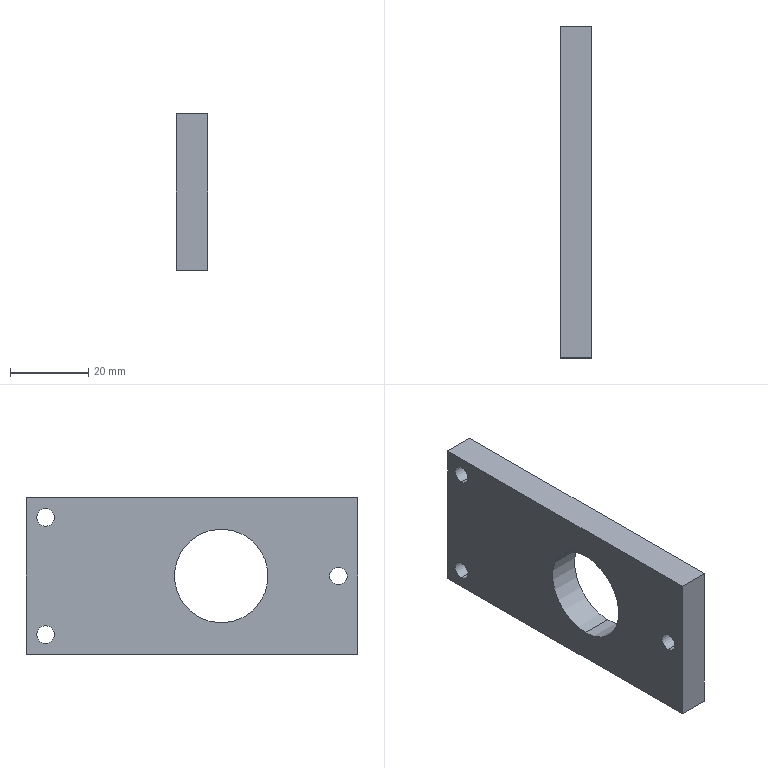Part | STEP file | 0243_213_Plate | 1 solid | 14 faces | box 8 x 85 x 40 mm | volume 23199 mm3 | cylinder 8 | plane 6 | commonest cylinder face diameters 4.5 x6 24 x2
STEP:
#1=CARTESIAN_POINT('',(0.,0.,0.));
#2=DIRECTION('',(0.,0.,1.));
#3=DIRECTION('',(1.,0.,0.));
#4=AXIS2_PLACEMENT_3D('',#1,#2,#3);
#5=CARTESIAN_POINT('',(0.,-80.,-2.25));
#6=VERTEX_POINT('',#5);
#7=CARTESIAN_POINT('',(8.,-80.,-2.25));
#8=VERTEX_POINT('',#7);
#9=CARTESIAN_POINT('',(8.,-80.,-2.25));
#10=DIRECTION('',(1.,0.,0.));
#11=VECTOR('',#10,1.);
#12=LINE('',#9,#11);
#13=CARTESIAN_POINT('',(8.,-80.,0.));
#14=DIRECTION('',(1.,0.,0.));
#15=DIRECTION('',(0.,0.,-1.));
#16=AXIS2_PLACEMENT_3D('',#13,#14,#15);
#17=CYLINDRICAL_SURFACE('',#16,2.25);
#18=CARTESIAN_POINT('',(6.283,0.));
#19=DIRECTION('',(0.,1.));
#20=VECTOR('',#19,1.);
#21=LINE('',#18,#20);
#22=(GEOMETRIC_REPRESENTATION_CONTEXT(2)PARAMETRIC_REPRESENTATION_CONTEXT()REPRESENTATION_CONTEXT('',''));
#23=DEFINITIONAL_REPRESENTATION('',(#21),#22);
#24=PCURVE('',#17,#23);
#25=CARTESIAN_POINT('',(8.,-80.,0.));
#26=DIRECTION('',(1.,0.,0.));
#27=DIRECTION('',(0.,0.,-1.));
#28=AXIS2_PLACEMENT_3D('',#25,#26,#27);
#29=CYLINDRICAL_SURFACE('',#28,2.25);
#30=CARTESIAN_POINT('',(0.,0.));
#31=DIRECTION('',(0.,1.));
#32=VECTOR('',#31,1.);
#33=LINE('',#30,#32);
#34=(GEOMETRIC_REPRESENTATION_CONTEXT(2)PARAMETRIC_REPRESENTATION_CONTEXT()REPRESENTATION_CONTEXT('',''));
#35=DEFINITIONAL_REPRESENTATION('',(#33),#34);
#36=PCURVE('',#29,#35);
#37=SURFACE_CURVE('',#12,(#24,#36),.PCURVE_S1.);
#38=EDGE_CURVE('',#6,#8,#37,.T.);
#39=ORIENTED_EDGE('',*,*,#38,.T.);
#40=CARTESIAN_POINT('',(8.,-80.,2.25));
#41=VERTEX_POINT('',#40);
#42=CARTESIAN_POINT('',(8.,-80.,0.));
#43=DIRECTION('',(1.,0.,0.));
#44=DIRECTION('',(0.,0.,-1.));
#45=AXIS2_PLACEMENT_3D('',#42,#43,#44);
#46=CIRCLE('',#45,2.25);
#47=CARTESIAN_POINT('',(0.,0.));
#48=DIRECTION('',(1.,0.));
#49=VECTOR('',#48,1.);
#50=LINE('',#47,#49);
#51=(GEOMETRIC_REPRESENTATION_CONTEXT(2)PARAMETRIC_REPRESENTATION_CONTEXT()REPRESENTATION_CONTEXT('',''));
#52=DEFINITIONAL_REPRESENTATION('',(#50),#51);
#53=PCURVE('',#17,#52);
#54=CARTESIAN_POINT('',(8.,0.,20.));
#55=DIRECTION('',(-1.,0.,0.));
#56=DIRECTION('',(0.,0.,1.));
#57=AXIS2_PLACEMENT_3D('',#54,#55,#56);
#58=PLANE('',#57);
#59=CARTESIAN_POINT('',(-22.25,-80.));
#60=CARTESIAN_POINT('',(-22.25,-76.103));
#61=CARTESIAN_POINT('',(-18.875,-78.051));
#62=CARTESIAN_POINT('',(-15.5,-80.));
#63=CARTESIAN_POINT('',(-18.875,-81.949));
#64=CARTESIAN_POINT('',(-22.25,-83.897));
#65=CARTESIAN_POINT('',(-22.25,-80.));
#66=(BOUNDED_CURVE()B_SPLINE_CURVE(2,(#59,#60,#61,#62,#63,#64,#65),.UNSPECIFIED.,.T.,.F.)B_SPLINE_CURVE_WITH_KNOTS((1,2,2,2,2,1),(-2.094,0.,2.094,4.189,6.283,8.378),.UNSPECIFIED.)CURVE()GEOMETRIC_REPRESENTATION_ITEM()RATIONAL_B_SPLINE_CURVE((1.,0.5,1.,0.5,1.,0.5,1.))REPRESENTATION_ITEM(''));
#67=(GEOMETRIC_REPRESENTATION_CONTEXT(2)PARAMETRIC_REPRESENTATION_CONTEXT()REPRESENTATION_CONTEXT('',''));
#68=DEFINITIONAL_REPRESENTATION('',(#66),#67);
#69=PCURVE('',#58,#68);
#70=SURFACE_CURVE('',#46,(#53,#69),.PCURVE_S1.);
#71=EDGE_CURVE('',#41,#8,#70,.T.);
#72=ORIENTED_EDGE('',*,*,#71,.F.);
#73=CARTESIAN_POINT('',(0.,-80.,2.25));
#74=VERTEX_POINT('',#73);
#75=CARTESIAN_POINT('',(8.,-80.,2.25));
#76=DIRECTION('',(1.,0.,0.));
#77=VECTOR('',#76,1.);
#78=LINE('',#75,#77);
#79=CARTESIAN_POINT('',(3.142,0.));
#80=DIRECTION('',(0.,1.));
#81=VECTOR('',#80,1.);
#82=LINE('',#79,#81);
#83=(GEOMETRIC_REPRESENTATION_CONTEXT(2)PARAMETRIC_REPRESENTATION_CONTEXT()REPRESENTATION_CONTEXT('',''));
#84=DEFINITIONAL_REPRESENTATION('',(#82),#83);
#85=PCURVE('',#17,#84);
#86=CARTESIAN_POINT('',(3.142,0.));
#87=DIRECTION('',(0.,1.));
#88=VECTOR('',#87,1.);
#89=LINE('',#86,#88);
#90=(GEOMETRIC_REPRESENTATION_CONTEXT(2)PARAMETRIC_REPRESENTATION_CONTEXT()REPRESENTATION_CONTEXT('',''));
#91=DEFINITIONAL_REPRESENTATION('',(#89),#90);
#92=PCURVE('',#29,#91);
#93=SURFACE_CURVE('',#78,(#85,#92),.PCURVE_S1.);
#94=EDGE_CURVE('',#74,#41,#93,.T.);
#95=ORIENTED_EDGE('',*,*,#94,.F.);
#96=CARTESIAN_POINT('',(0.,-80.,0.));
#97=DIRECTION('',(1.,0.,0.));
#98=DIRECTION('',(0.,0.,-1.));
#99=AXIS2_PLACEMENT_3D('',#96,#97,#98);
#100=CIRCLE('',#99,2.25);
#101=CARTESIAN_POINT('',(0.,-8.));
#102=DIRECTION('',(1.,0.));
#103=VECTOR('',#102,1.);
#104=LINE('',#101,#103);
#105=(GEOMETRIC_REPRESENTATION_CONTEXT(2)PARAMETRIC_REPRESENTATION_CONTEXT()REPRESENTATION_CONTEXT('',''));
#106=DEFINITIONAL_REPRESENTATION('',(#104),#105);
#107=PCURVE('',#17,#106);
#108=CARTESIAN_POINT('',(0.,0.,20.));
#109=DIRECTION('',(-1.,0.,0.));
#110=DIRECTION('',(0.,0.,1.));
#111=AXIS2_PLACEMENT_3D('',#108,#109,#110);
#112=PLANE('',#111);
#113=CARTESIAN_POINT('',(-22.25,-80.));
#114=CARTESIAN_POINT('',(-22.25,-76.103));
#115=CARTESIAN_POINT('',(-18.875,-78.051));
#116=CARTESIAN_POINT('',(-15.5,-80.));
#117=CARTESIAN_POINT('',(-18.875,-81.949));
#118=CARTESIAN_POINT('',(-22.25,-83.897));
#119=CARTESIAN_POINT('',(-22.25,-80.));
#120=(BOUNDED_CURVE()B_SPLINE_CURVE(2,(#113,#114,#115,#116,#117,#118,#119),.UNSPECIFIED.,.T.,.F.)B_SPLINE_CURVE_WITH_KNOTS((1,2,2,2,2,1),(-2.094,0.,2.094,4.189,6.283,8.378),.UNSPECIFIED.)CURVE()GEOMETRIC_REPRESENTATION_ITEM()RATIONAL_B_SPLINE_CURVE((1.,0.5,1.,0.5,1.,0.5,1.))REPRESENTATION_ITEM(''));
#121=(GEOMETRIC_REPRESENTATION_CONTEXT(2)PARAMETRIC_REPRESENTATION_CONTEXT()REPRESENTATION_CONTEXT('',''));
#122=DEFINITIONAL_REPRESENTATION('',(#120),#121);
#123=PCURVE('',#112,#122);
#124=SURFACE_CURVE('',#100,(#107,#123),.PCURVE_S1.);
#125=EDGE_CURVE('',#74,#6,#124,.T.);
#126=ORIENTED_EDGE('',*,*,#125,.T.);
#127=EDGE_LOOP('',(#39,#72,#95,#126));
#128=FACE_BOUND('',#127,.F.);
#129=ADVANCED_FACE('',(#128),#17,.F.);
#130=CARTESIAN_POINT('',(0.,-5.,12.75));
#131=VERTEX_POINT('',#130);
#132=CARTESIAN_POINT('',(8.,-5.,12.75));
#133=VERTEX_POINT('',#132);
#134=CARTESIAN_POINT('',(8.,-5.,12.75));
#135=DIRECTION('',(1.,0.,0.));
#136=VECTOR('',#135,1.);
#137=LINE('',#134,#136);
#138=CARTESIAN_POINT('',(8.,-5.,15.));
#139=DIRECTION('',(1.,0.,0.));
#140=DIRECTION('',(0.,0.,-1.));
#141=AXIS2_PLACEMENT_3D('',#138,#139,#140);
#142=CYLINDRICAL_SURFACE('',#141,2.25);
#143=CARTESIAN_POINT('',(6.283,0.));
#144=DIRECTION('',(0.,1.));
#145=VECTOR('',#144,1.);
#146=LINE('',#143,#145);
#147=(GEOMETRIC_REPRESENTATION_CONTEXT(2)PARAMETRIC_REPRESENTATION_CONTEXT()REPRESENTATION_CONTEXT('',''));
#148=DEFINITIONAL_REPRESENTATION('',(#146),#147);
#149=PCURVE('',#142,#148);
#150=CARTESIAN_POINT('',(8.,-5.,15.));
#151=DIRECTION('',(1.,0.,0.));
#152=DIRECTION('',(0.,0.,-1.));
#153=AXIS2_PLACEMENT_3D('',#150,#151,#152);
#154=CYLINDRICAL_SURFACE('',#153,2.25);
#155=CARTESIAN_POINT('',(0.,0.));
#156=DIRECTION('',(0.,1.));
#157=VECTOR('',#156,1.);
#158=LINE('',#155,#157);
#159=(GEOMETRIC_REPRESENTATION_CONTEXT(2)PARAMETRIC_REPRESENTATION_CONTEXT()REPRESENTATION_CONTEXT('',''));
#160=DEFINITIONAL_REPRESENTATION('',(#158),#159);
#161=PCURVE('',#154,#160);
#162=SURFACE_CURVE('',#137,(#149,#161),.PCURVE_S1.);
#163=EDGE_CURVE('',#131,#133,#162,.T.);
#164=ORIENTED_EDGE('',*,*,#163,.T.);
#165=CARTESIAN_POINT('',(8.,-5.,17.25));
#166=VERTEX_POINT('',#165);
#167=CARTESIAN_POINT('',(8.,-5.,15.));
#168=DIRECTION('',(1.,0.,0.));
#169=DIRECTION('',(0.,0.,-1.));
#170=AXIS2_PLACEMENT_3D('',#167,#168,#169);
#171=CIRCLE('',#170,2.25);
#172=CARTESIAN_POINT('',(0.,0.));
#173=DIRECTION('',(1.,0.));
#174=VECTOR('',#173,1.);
#175=LINE('',#172,#174);
#176=(GEOMETRIC_REPRESENTATION_CONTEXT(2)PARAMETRIC_REPRESENTATION_CONTEXT()REPRESENTATION_CONTEXT('',''));
#177=DEFINITIONAL_REPRESENTATION('',(#175),#176);
#178=PCURVE('',#142,#177);
#179=CARTESIAN_POINT('',(-7.25,-5.));
#180=CARTESIAN_POINT('',(-7.25,-1.103));
#181=CARTESIAN_POINT('',(-3.875,-3.051));
#182=CARTESIAN_POINT('',(-0.5,-5.));
#183=CARTESIAN_POINT('',(-3.875,-6.949));
#184=CARTESIAN_POINT('',(-7.25,-8.897));
#185=CARTESIAN_POINT('',(-7.25,-5.));
#186=(BOUNDED_CURVE()B_SPLINE_CURVE(2,(#179,#180,#181,#182,#183,#184,#185),.UNSPECIFIED.,.T.,.F.)B_SPLINE_CURVE_WITH_KNOTS((1,2,2,2,2,1),(-2.094,0.,2.094,4.189,6.283,8.378),.UNSPECIFIED.)CURVE()GEOMETRIC_REPRESENTATION_ITEM()RATIONAL_B_SPLINE_CURVE((1.,0.5,1.,0.5,1.,0.5,1.))REPRESENTATION_ITEM(''));
#187=(GEOMETRIC_REPRESENTATION_CONTEXT(2)PARAMETRIC_REPRESENTATION_CONTEXT()REPRESENTATION_CONTEXT('',''));
#188=DEFINITIONAL_REPRESENTATION('',(#186),#187);
#189=PCURVE('',#58,#188);
#190=SURFACE_CURVE('',#171,(#178,#189),.PCURVE_S1.);
#191=EDGE_CURVE('',#166,#133,#190,.T.);
#192=ORIENTED_EDGE('',*,*,#191,.F.);
#193=CARTESIAN_POINT('',(0.,-5.,17.25));
#194=VERTEX_POINT('',#193);
#195=CARTESIAN_POINT('',(8.,-5.,17.25));
#196=DIRECTION('',(1.,0.,0.));
#197=VECTOR('',#196,1.);
#198=LINE('',#195,#197);
#199=CARTESIAN_POINT('',(3.142,0.));
#200=DIRECTION('',(0.,1.));
#201=VECTOR('',#200,1.);
#202=LINE('',#199,#201);
#203=(GEOMETRIC_REPRESENTATION_CONTEXT(2)PARAMETRIC_REPRESENTATION_CONTEXT()REPRESENTATION_CONTEXT('',''));
#204=DEFINITIONAL_REPRESENTATION('',(#202),#203);
#205=PCURVE('',#142,#204);
#206=CARTESIAN_POINT('',(3.142,0.));
#207=DIRECTION('',(0.,1.));
#208=VECTOR('',#207,1.);
#209=LINE('',#206,#208);
#210=(GEOMETRIC_REPRESENTATION_CONTEXT(2)PARAMETRIC_REPRESENTATION_CONTEXT()REPRESENTATION_CONTEXT('',''));
#211=DEFINITIONAL_REPRESENTATION('',(#209),#210);
#212=PCURVE('',#154,#211);
#213=SURFACE_CURVE('',#198,(#205,#212),.PCURVE_S1.);
#214=EDGE_CURVE('',#194,#166,#213,.T.);
#215=ORIENTED_EDGE('',*,*,#214,.F.);
#216=CARTESIAN_POINT('',(0.,-5.,15.));
#217=DIRECTION('',(1.,0.,0.));
#218=DIRECTION('',(0.,0.,-1.));
#219=AXIS2_PLACEMENT_3D('',#216,#217,#218);
#220=CIRCLE('',#219,2.25);
#221=CARTESIAN_POINT('',(0.,-8.));
#222=DIRECTION('',(1.,0.));
#223=VECTOR('',#222,1.);
#224=LINE('',#221,#223);
#225=(GEOMETRIC_REPRESENTATION_CONTEXT(2)PARAMETRIC_REPRESENTATION_CONTEXT()REPRESENTATION_CONTEXT('',''));
#226=DEFINITIONAL_REPRESENTATION('',(#224),#225);
#227=PCURVE('',#142,#226);
#228=CARTESIAN_POINT('',(-7.25,-5.));
#229=CARTESIAN_POINT('',(-7.25,-1.103));
#230=CARTESIAN_POINT('',(-3.875,-3.051));
#231=CARTESIAN_POINT('',(-0.5,-5.));
#232=CARTESIAN_POINT('',(-3.875,-6.949));
#233=CARTESIAN_POINT('',(-7.25,-8.897));
#234=CARTESIAN_POINT('',(-7.25,-5.));
#235=(BOUNDED_CURVE()B_SPLINE_CURVE(2,(#228,#229,#230,#231,#232,#233,#234),.UNSPECIFIED.,.T.,.F.)B_SPLINE_CURVE_WITH_KNOTS((1,2,2,2,2,1),(-2.094,0.,2.094,4.189,6.283,8.378),.UNSPECIFIED.)CURVE()GEOMETRIC_REPRESENTATION_ITEM()RATIONAL_B_SPLINE_CURVE((1.,0.5,1.,0.5,1.,0.5,1.))REPRESENTATION_ITEM(''));
#236=(GEOMETRIC_REPRESENTATION_CONTEXT(2)PARAMETRIC_REPRESENTATION_CONTEXT()REPRESENTATION_CONTEXT('',''));
#237=DEFINITIONAL_REPRESENTATION('',(#235),#236);
#238=PCURVE('',#112,#237);
#239=SURFACE_CURVE('',#220,(#227,#238),.PCURVE_S1.);
#240=EDGE_CURVE('',#194,#131,#239,.T.);
#241=ORIENTED_EDGE('',*,*,#240,.T.);
#242=EDGE_LOOP('',(#164,#192,#215,#241));
#243=FACE_BOUND('',#242,.F.);
#244=ADVANCED_FACE('',(#243),#142,.F.);
#245=CARTESIAN_POINT('',(0.,-5.,-17.25));
#246=VERTEX_POINT('',#245);
#247=CARTESIAN_POINT('',(8.,-5.,-17.25));
#248=VERTEX_POINT('',#247);
#249=CARTESIAN_POINT('',(8.,-5.,-17.25));
#250=DIRECTION('',(1.,0.,0.));
#251=VECTOR('',#250,1.);
#252=LINE('',#249,#251);
#253=CARTESIAN_POINT('',(8.,-5.,-15.));
#254=DIRECTION('',(1.,0.,0.));
#255=DIRECTION('',(0.,0.,-1.));
#256=AXIS2_PLACEMENT_3D('',#253,#254,#255);
#257=CYLINDRICAL_SURFACE('',#256,2.25);
#258=CARTESIAN_POINT('',(6.283,0.));
#259=DIRECTION('',(0.,1.));
#260=VECTOR('',#259,1.);
#261=LINE('',#258,#260);
#262=(GEOMETRIC_REPRESENTATION_CONTEXT(2)PARAMETRIC_REPRESENTATION_CONTEXT()REPRESENTATION_CONTEXT('',''));
#263=DEFINITIONAL_REPRESENTATION('',(#261),#262);
#264=PCURVE('',#257,#263);
#265=CARTESIAN_POINT('',(8.,-5.,-15.));
#266=DIRECTION('',(1.,0.,0.));
#267=DIRECTION('',(0.,0.,-1.));
#268=AXIS2_PLACEMENT_3D('',#265,#266,#267);
#269=CYLINDRICAL_SURFACE('',#268,2.25);
#270=CARTESIAN_POINT('',(0.,0.));
#271=DIRECTION('',(0.,1.));
#272=VECTOR('',#271,1.);
#273=LINE('',#270,#272);
#274=(GEOMETRIC_REPRESENTATION_CONTEXT(2)PARAMETRIC_REPRESENTATION_CONTEXT()REPRESENTATION_CONTEXT('',''));
#275=DEFINITIONAL_REPRESENTATION('',(#273),#274);
#276=PCURVE('',#269,#275);
#277=SURFACE_CURVE('',#252,(#264,#276),.PCURVE_S1.);
#278=EDGE_CURVE('',#246,#248,#277,.T.);
#279=ORIENTED_EDGE('',*,*,#278,.T.);
#280=CARTESIAN_POINT('',(8.,-5.,-12.75));
#281=VERTEX_POINT('',#280);
#282=CARTESIAN_POINT('',(8.,-5.,-15.));
#283=DIRECTION('',(1.,0.,0.));
#284=DIRECTION('',(0.,0.,-1.));
#285=AXIS2_PLACEMENT_3D('',#282,#283,#284);
#286=CIRCLE('',#285,2.25);
#287=CARTESIAN_POINT('',(0.,0.));
#288=DIRECTION('',(1.,0.));
#289=VECTOR('',#288,1.);
#290=LINE('',#287,#289);
#291=(GEOMETRIC_REPRESENTATION_CONTEXT(2)PARAMETRIC_REPRESENTATION_CONTEXT()REPRESENTATION_CONTEXT('',''));
#292=DEFINITIONAL_REPRESENTATION('',(#290),#291);
#293=PCURVE('',#257,#292);
#294=CARTESIAN_POINT('',(-37.25,-5.));
#295=CARTESIAN_POINT('',(-37.25,-1.103));
#296=CARTESIAN_POINT('',(-33.875,-3.051));
#297=CARTESIAN_POINT('',(-30.5,-5.));
#298=CARTESIAN_POINT('',(-33.875,-6.949));
#299=CARTESIAN_POINT('',(-37.25,-8.897));
#300=CARTESIAN_POINT('',(-37.25,-5.));
#301=(BOUNDED_CURVE()B_SPLINE_CURVE(2,(#294,#295,#296,#297,#298,#299,#300),.UNSPECIFIED.,.T.,.F.)B_SPLINE_CURVE_WITH_KNOTS((1,2,2,2,2,1),(-2.094,0.,2.094,4.189,6.283,8.378),.UNSPECIFIED.)CURVE()GEOMETRIC_REPRESENTATION_ITEM()RATIONAL_B_SPLINE_CURVE((1.,0.5,1.,0.5,1.,0.5,1.))REPRESENTATION_ITEM(''));
#302=(GEOMETRIC_REPRESENTATION_CONTEXT(2)PARAMETRIC_REPRESENTATION_CONTEXT()REPRESENTATION_CONTEXT('',''));
#303=DEFINITIONAL_REPRESENTATION('',(#301),#302);
#304=PCURVE('',#58,#303);
#305=SURFACE_CURVE('',#286,(#293,#304),.PCURVE_S1.);
#306=EDGE_CURVE('',#281,#248,#305,.T.);
#307=ORIENTED_EDGE('',*,*,#306,.F.);
#308=CARTESIAN_POINT('',(0.,-5.,-12.75));
#309=VERTEX_POINT('',#308);
#310=CARTESIAN_POINT('',(8.,-5.,-12.75));
#311=DIRECTION('',(1.,0.,0.));
#312=VECTOR('',#311,1.);
#313=LINE('',#310,#312);
#314=CARTESIAN_POINT('',(3.142,0.));
#315=DIRECTION('',(0.,1.));
#316=VECTOR('',#315,1.);
#317=LINE('',#314,#316);
#318=(GEOMETRIC_REPRESENTATION_CONTEXT(2)PARAMETRIC_REPRESENTATION_CONTEXT()REPRESENTATION_CONTEXT('',''));
#319=DEFINITIONAL_REPRESENTATION('',(#317),#318);
#320=PCURVE('',#257,#319);
#321=CARTESIAN_POINT('',(3.142,0.));
#322=DIRECTION('',(0.,1.));
#323=VECTOR('',#322,1.);
#324=LINE('',#321,#323);
#325=(GEOMETRIC_REPRESENTATION_CONTEXT(2)PARAMETRIC_REPRESENTATION_CONTEXT()REPRESENTATION_CONTEXT('',''));
#326=DEFINITIONAL_REPRESENTATION('',(#324),#325);
#327=PCURVE('',#269,#326);
#328=SURFACE_CURVE('',#313,(#320,#327),.PCURVE_S1.);
#329=EDGE_CURVE('',#309,#281,#328,.T.);
#330=ORIENTED_EDGE('',*,*,#329,.F.);
#331=CARTESIAN_POINT('',(0.,-5.,-15.));
#332=DIRECTION('',(1.,0.,0.));
#333=DIRECTION('',(0.,0.,-1.));
#334=AXIS2_PLACEMENT_3D('',#331,#332,#333);
#335=CIRCLE('',#334,2.25);
#336=CARTESIAN_POINT('',(0.,-8.));
#337=DIRECTION('',(1.,0.));
#338=VECTOR('',#337,1.);
#339=LINE('',#336,#338);
#340=(GEOMETRIC_REPRESENTATION_CONTEXT(2)PARAMETRIC_REPRESENTATION_CONTEXT()REPRESENTATION_CONTEXT('',''));
#341=DEFINITIONAL_REPRESENTATION('',(#339),#340);
#342=PCURVE('',#257,#341);
#343=CARTESIAN_POINT('',(-37.25,-5.));
#344=CARTESIAN_POINT('',(-37.25,-1.103));
#345=CARTESIAN_POINT('',(-33.875,-3.051));
#346=CARTESIAN_POINT('',(-30.5,-5.));
#347=CARTESIAN_POINT('',(-33.875,-6.949));
#348=CARTESIAN_POINT('',(-37.25,-8.897));
#349=CARTESIAN_POINT('',(-37.25,-5.));
#350=(BOUNDED_CURVE()B_SPLINE_CURVE(2,(#343,#344,#345,#346,#347,#348,#349),.UNSPECIFIED.,.T.,.F.)B_SPLINE_CURVE_WITH_KNOTS((1,2,2,2,2,1),(-2.094,0.,2.094,4.189,6.283,8.378),.UNSPECIFIED.)CURVE()GEOMETRIC_REPRESENTATION_ITEM()RATIONAL_B_SPLINE_CURVE((1.,0.5,1.,0.5,1.,0.5,1.))REPRESENTATION_ITEM(''));
#351=(GEOMETRIC_REPRESENTATION_CONTEXT(2)PARAMETRIC_REPRESENTATION_CONTEXT()REPRESENTATION_CONTEXT('',''));
#352=DEFINITIONAL_REPRESENTATION('',(#350),#351);
#353=PCURVE('',#112,#352);
#354=SURFACE_CURVE('',#335,(#342,#353),.PCURVE_S1.);
#355=EDGE_CURVE('',#309,#246,#354,.T.);
#356=ORIENTED_EDGE('',*,*,#355,.T.);
#357=EDGE_LOOP('',(#279,#307,#330,#356));
#358=FACE_BOUND('',#357,.F.);
#359=ADVANCED_FACE('',(#358),#257,.F.);
#360=CARTESIAN_POINT('',(0.,-50.,-12.));
#361=VERTEX_POINT('',#360);
#362=CARTESIAN_POINT('',(8.,-50.,-12.));
#363=VERTEX_POINT('',#362);
#364=CARTESIAN_POINT('',(0.,-50.,-12.));
#365=DIRECTION('',(1.,0.,0.));
#366=VECTOR('',#365,1.);
#367=LINE('',#364,#366);
#368=CARTESIAN_POINT('',(0.,-50.,0.));
#369=DIRECTION('',(1.,0.,0.));
#370=DIRECTION('',(0.,0.,-1.));
#371=AXIS2_PLACEMENT_3D('',#368,#369,#370);
#372=CYLINDRICAL_SURFACE('',#371,12.);
#373=CARTESIAN_POINT('',(6.283,0.));
#374=DIRECTION('',(0.,1.));
#375=VECTOR('',#374,1.);
#376=LINE('',#373,#375);
#377=(GEOMETRIC_REPRESENTATION_CONTEXT(2)PARAMETRIC_REPRESENTATION_CONTEXT()REPRESENTATION_CONTEXT('',''));
#378=DEFINITIONAL_REPRESENTATION('',(#376),#377);
#379=PCURVE('',#372,#378);
#380=CARTESIAN_POINT('',(0.,-50.,0.));
#381=DIRECTION('',(1.,0.,0.));
#382=DIRECTION('',(0.,0.,-1.));
#383=AXIS2_PLACEMENT_3D('',#380,#381,#382);
#384=CYLINDRICAL_SURFACE('',#383,12.);
#385=CARTESIAN_POINT('',(0.,0.));
#386=DIRECTION('',(0.,1.));
#387=VECTOR('',#386,1.);
#388=LINE('',#385,#387);
#389=(GEOMETRIC_REPRESENTATION_CONTEXT(2)PARAMETRIC_REPRESENTATION_CONTEXT()REPRESENTATION_CONTEXT('',''));
#390=DEFINITIONAL_REPRESENTATION('',(#388),#389);
#391=PCURVE('',#384,#390);
#392=SURFACE_CURVE('',#367,(#379,#391),.PCURVE_S1.);
#393=EDGE_CURVE('',#361,#363,#392,.T.);
#394=ORIENTED_EDGE('',*,*,#393,.T.);
#395=CARTESIAN_POINT('',(8.,-50.,12.));
#396=VERTEX_POINT('',#395);
#397=CARTESIAN_POINT('',(8.,-50.,0.));
#398=DIRECTION('',(1.,0.,0.));
#399=DIRECTION('',(0.,0.,-1.));
#400=AXIS2_PLACEMENT_3D('',#397,#398,#399);
#401=CIRCLE('',#400,12.);
#402=CARTESIAN_POINT('',(0.,8.));
#403=DIRECTION('',(1.,0.));
#404=VECTOR('',#403,1.);
#405=LINE('',#402,#404);
#406=(GEOMETRIC_REPRESENTATION_CONTEXT(2)PARAMETRIC_REPRESENTATION_CONTEXT()REPRESENTATION_CONTEXT('',''));
#407=DEFINITIONAL_REPRESENTATION('',(#405),#406);
#408=PCURVE('',#372,#407);
#409=CARTESIAN_POINT('',(-32.,-50.));
#410=CARTESIAN_POINT('',(-32.,-29.215));
#411=CARTESIAN_POINT('',(-14.,-39.608));
#412=CARTESIAN_POINT('',(4.,-50.));
#413=CARTESIAN_POINT('',(-14.,-60.392));
#414=CARTESIAN_POINT('',(-32.,-70.785));
#415=CARTESIAN_POINT('',(-32.,-50.));
#416=(BOUNDED_CURVE()B_SPLINE_CURVE(2,(#409,#410,#411,#412,#413,#414,#415),.UNSPECIFIED.,.T.,.F.)B_SPLINE_CURVE_WITH_KNOTS((1,2,2,2,2,1),(-2.094,0.,2.094,4.189,6.283,8.378),.UNSPECIFIED.)CURVE()GEOMETRIC_REPRESENTATION_ITEM()RATIONAL_B_SPLINE_CURVE((1.,0.5,1.,0.5,1.,0.5,1.))REPRESENTATION_ITEM(''));
#417=(GEOMETRIC_REPRESENTATION_CONTEXT(2)PARAMETRIC_REPRESENTATION_CONTEXT()REPRESENTATION_CONTEXT('',''));
#418=DEFINITIONAL_REPRESENTATION('',(#416),#417);
#419=PCURVE('',#58,#418);
#420=SURFACE_CURVE('',#401,(#408,#419),.PCURVE_S1.);
#421=EDGE_CURVE('',#396,#363,#420,.T.);
#422=ORIENTED_EDGE('',*,*,#421,.F.);
#423=CARTESIAN_POINT('',(0.,-50.,12.));
#424=VERTEX_POINT('',#423);
#425=CARTESIAN_POINT('',(0.,-50.,12.));
#426=DIRECTION('',(1.,0.,0.));
#427=VECTOR('',#426,1.);
#428=LINE('',#425,#427);
#429=CARTESIAN_POINT('',(3.142,0.));
#430=DIRECTION('',(0.,1.));
#431=VECTOR('',#430,1.);
#432=LINE('',#429,#431);
#433=(GEOMETRIC_REPRESENTATION_CONTEXT(2)PARAMETRIC_REPRESENTATION_CONTEXT()REPRESENTATION_CONTEXT('',''));
#434=DEFINITIONAL_REPRESENTATION('',(#432),#433);
#435=PCURVE('',#372,#434);
#436=CARTESIAN_POINT('',(3.142,0.));
#437=DIRECTION('',(0.,1.));
#438=VECTOR('',#437,1.);
#439=LINE('',#436,#438);
#440=(GEOMETRIC_REPRESENTATION_CONTEXT(2)PARAMETRIC_REPRESENTATION_CONTEXT()REPRESENTATION_CONTEXT('',''));
#441=DEFINITIONAL_REPRESENTATION('',(#439),#440);
#442=PCURVE('',#384,#441);
#443=SURFACE_CURVE('',#428,(#435,#442),.PCURVE_S1.);
#444=EDGE_CURVE('',#424,#396,#443,.T.);
#445=ORIENTED_EDGE('',*,*,#444,.F.);
#446=CARTESIAN_POINT('',(0.,-50.,0.));
#447=DIRECTION('',(1.,0.,0.));
#448=DIRECTION('',(0.,0.,-1.));
#449=AXIS2_PLACEMENT_3D('',#446,#447,#448);
#450=CIRCLE('',#449,12.);
#451=CARTESIAN_POINT('',(0.,0.));
#452=DIRECTION('',(1.,0.));
#453=VECTOR('',#452,1.);
#454=LINE('',#451,#453);
#455=(GEOMETRIC_REPRESENTATION_CONTEXT(2)PARAMETRIC_REPRESENTATION_CONTEXT()REPRESENTATION_CONTEXT('',''));
#456=DEFINITIONAL_REPRESENTATION('',(#454),#455);
#457=PCURVE('',#372,#456);
#458=CARTESIAN_POINT('',(-32.,-50.));
#459=CARTESIAN_POINT('',(-32.,-29.215));
#460=CARTESIAN_POINT('',(-14.,-39.608));
#461=CARTESIAN_POINT('',(4.,-50.));
#462=CARTESIAN_POINT('',(-14.,-60.392));
#463=CARTESIAN_POINT('',(-32.,-70.785));
#464=CARTESIAN_POINT('',(-32.,-50.));
#465=(BOUNDED_CURVE()B_SPLINE_CURVE(2,(#458,#459,#460,#461,#462,#463,#464),.UNSPECIFIED.,.T.,.F.)B_SPLINE_CURVE_WITH_KNOTS((1,2,2,2,2,1),(-2.094,0.,2.094,4.189,6.283,8.378),.UNSPECIFIED.)CURVE()GEOMETRIC_REPRESENTATION_ITEM()RATIONAL_B_SPLINE_CURVE((1.,0.5,1.,0.5,1.,0.5,1.))REPRESENTATION_ITEM(''));
#466=(GEOMETRIC_REPRESENTATION_CONTEXT(2)PARAMETRIC_REPRESENTATION_CONTEXT()REPRESENTATION_CONTEXT('',''));
#467=DEFINITIONAL_REPRESENTATION('',(#465),#466);
#468=PCURVE('',#112,#467);
#469=SURFACE_CURVE('',#450,(#457,#468),.PCURVE_S1.);
#470=EDGE_CURVE('',#424,#361,#469,.T.);
#471=ORIENTED_EDGE('',*,*,#470,.T.);
#472=EDGE_LOOP('',(#394,#422,#445,#471));
#473=FACE_BOUND('',#472,.F.);
#474=ADVANCED_FACE('',(#473),#372,.F.);
#475=CARTESIAN_POINT('',(0.,0.,20.));
#476=VERTEX_POINT('',#475);
#477=CARTESIAN_POINT('',(0.,-85.,20.));
#478=VERTEX_POINT('',#477);
#479=CARTESIAN_POINT('',(0.,-85.,20.));
#480=DIRECTION('',(0.,-1.,0.));
#481=VECTOR('',#480,1.);
#482=LINE('',#479,#481);
#483=CARTESIAN_POINT('',(8.,-85.,20.));
#484=DIRECTION('',(0.,0.,-1.));
#485=DIRECTION('',(0.,1.,0.));
#486=AXIS2_PLACEMENT_3D('',#483,#484,#485);
#487=PLANE('',#486);
#488=CARTESIAN_POINT('',(0.,-8.));
#489=DIRECTION('',(-1.,0.));
#490=VECTOR('',#489,1.);
#491=LINE('',#488,#490);
#492=(GEOMETRIC_REPRESENTATION_CONTEXT(2)PARAMETRIC_REPRESENTATION_CONTEXT()REPRESENTATION_CONTEXT('',''));
#493=DEFINITIONAL_REPRESENTATION('',(#491),#492);
#494=PCURVE('',#487,#493);
#495=CARTESIAN_POINT('',(0.,-85.));
#496=DIRECTION('',(0.,-1.));
#497=VECTOR('',#496,1.);
#498=LINE('',#495,#497);
#499=(GEOMETRIC_REPRESENTATION_CONTEXT(2)PARAMETRIC_REPRESENTATION_CONTEXT()REPRESENTATION_CONTEXT('',''));
#500=DEFINITIONAL_REPRESENTATION('',(#498),#499);
#501=PCURVE('',#112,#500);
#502=SURFACE_CURVE('',#482,(#494,#501),.PCURVE_S1.);
#503=EDGE_CURVE('',#476,#478,#502,.T.);
#504=ORIENTED_EDGE('',*,*,#503,.T.);
#505=CARTESIAN_POINT('',(8.,-85.,20.));
#506=VERTEX_POINT('',#505);
#507=CARTESIAN_POINT('',(8.,-85.,20.));
#508=DIRECTION('',(-1.,0.,0.));
#509=VECTOR('',#508,1.);
#510=LINE('',#507,#509);
#511=CARTESIAN_POINT('',(0.,0.));
#512=DIRECTION('',(0.,-1.));
#513=VECTOR('',#512,1.);
#514=LINE('',#511,#513);
#515=(GEOMETRIC_REPRESENTATION_CONTEXT(2)PARAMETRIC_REPRESENTATION_CONTEXT()REPRESENTATION_CONTEXT('',''));
#516=DEFINITIONAL_REPRESENTATION('',(#514),#515);
#517=PCURVE('',#487,#516);
#518=CARTESIAN_POINT('',(8.,-85.,20.));
#519=DIRECTION('',(0.,1.,0.));
#520=DIRECTION('',(0.,0.,1.));
#521=AXIS2_PLACEMENT_3D('',#518,#519,#520);
#522=PLANE('',#521);
#523=CARTESIAN_POINT('',(0.,0.));
#524=DIRECTION('',(0.,-1.));
#525=VECTOR('',#524,1.);
#526=LINE('',#523,#525);
#527=(GEOMETRIC_REPRESENTATION_CONTEXT(2)PARAMETRIC_REPRESENTATION_CONTEXT()REPRESENTATION_CONTEXT('',''));
#528=DEFINITIONAL_REPRESENTATION('',(#526),#527);
#529=PCURVE('',#522,#528);
#530=SURFACE_CURVE('',#510,(#517,#529),.PCURVE_S1.);
#531=EDGE_CURVE('',#506,#478,#530,.T.);
#532=ORIENTED_EDGE('',*,*,#531,.F.);
#533=CARTESIAN_POINT('',(8.,0.,20.));
#534=VERTEX_POINT('',#533);
#535=CARTESIAN_POINT('',(8.,-85.,20.));
#536=DIRECTION('',(0.,-1.,0.));
#537=VECTOR('',#536,1.);
#538=LINE('',#535,#537);
#539=CARTESIAN_POINT('',(0.,0.));
#540=DIRECTION('',(-1.,0.));
#541=VECTOR('',#540,1.);
#542=LINE('',#539,#541);
#543=(GEOMETRIC_REPRESENTATION_CONTEXT(2)PARAMETRIC_REPRESENTATION_CONTEXT()REPRESENTATION_CONTEXT('',''));
#544=DEFINITIONAL_REPRESENTATION('',(#542),#543);
#545=PCURVE('',#487,#544);
#546=CARTESIAN_POINT('',(0.,-85.));
#547=DIRECTION('',(0.,-1.));
#548=VECTOR('',#547,1.);
#549=LINE('',#546,#548);
#550=(GEOMETRIC_REPRESENTATION_CONTEXT(2)PARAMETRIC_REPRESENTATION_CONTEXT()REPRESENTATION_CONTEXT('',''));
#551=DEFINITIONAL_REPRESENTATION('',(#549),#550);
#552=PCURVE('',#58,#551);
#553=SURFACE_CURVE('',#538,(#545,#552),.PCURVE_S1.);
#554=EDGE_CURVE('',#534,#506,#553,.T.);
#555=ORIENTED_EDGE('',*,*,#554,.F.);
#556=CARTESIAN_POINT('',(8.,0.,20.));
#557=DIRECTION('',(-1.,0.,0.));
#558=VECTOR('',#557,1.);
#559=LINE('',#556,#558);
#560=CARTESIAN_POINT('',(85.,0.));
#561=DIRECTION('',(0.,-1.));
#562=VECTOR('',#561,1.);
#563=LINE('',#560,#562);
#564=(GEOMETRIC_REPRESENTATION_CONTEXT(2)PARAMETRIC_REPRESENTATION_CONTEXT()REPRESENTATION_CONTEXT('',''));
#565=DEFINITIONAL_REPRESENTATION('',(#563),#564);
#566=PCURVE('',#487,#565);
#567=CARTESIAN_POINT('',(8.,0.,20.));
#568=DIRECTION('',(0.,-1.,0.));
#569=DIRECTION('',(0.,0.,-1.));
#570=AXIS2_PLACEMENT_3D('',#567,#568,#569);
#571=PLANE('',#570);
#572=CARTESIAN_POINT('',(0.,0.));
#573=DIRECTION('',(0.,-1.));
#574=VECTOR('',#573,1.);
#575=LINE('',#572,#574);
#576=(GEOMETRIC_REPRESENTATION_CONTEXT(2)PARAMETRIC_REPRESENTATION_CONTEXT()REPRESENTATION_CONTEXT('',''));
#577=DEFINITIONAL_REPRESENTATION('',(#575),#576);
#578=PCURVE('',#571,#577);
#579=SURFACE_CURVE('',#559,(#566,#578),.PCURVE_S1.);
#580=EDGE_CURVE('',#534,#476,#579,.T.);
#581=ORIENTED_EDGE('',*,*,#580,.T.);
#582=EDGE_LOOP('',(#504,#532,#555,#581));
#583=FACE_BOUND('',#582,.T.);
#584=ADVANCED_FACE('',(#583),#487,.F.);
#585=CARTESIAN_POINT('',(0.,-85.,-20.));
#586=VERTEX_POINT('',#585);
#587=CARTESIAN_POINT('',(0.,-85.,20.));
#588=DIRECTION('',(0.,0.,-1.));
#589=VECTOR('',#588,1.);
#590=LINE('',#587,#589);
#591=CARTESIAN_POINT('',(0.,-8.));
#592=DIRECTION('',(-1.,0.));
#593=VECTOR('',#592,1.);
#594=LINE('',#591,#593);
#595=(GEOMETRIC_REPRESENTATION_CONTEXT(2)PARAMETRIC_REPRESENTATION_CONTEXT()REPRESENTATION_CONTEXT('',''));
#596=DEFINITIONAL_REPRESENTATION('',(#594),#595);
#597=PCURVE('',#522,#596);
#598=CARTESIAN_POINT('',(0.,-85.));
#599=DIRECTION('',(-1.,0.));
#600=VECTOR('',#599,1.);
#601=LINE('',#598,#600);
#602=(GEOMETRIC_REPRESENTATION_CONTEXT(2)PARAMETRIC_REPRESENTATION_CONTEXT()REPRESENTATION_CONTEXT('',''));
#603=DEFINITIONAL_REPRESENTATION('',(#601),#602);
#604=PCURVE('',#112,#603);
#605=SURFACE_CURVE('',#590,(#597,#604),.PCURVE_S1.);
#606=EDGE_CURVE('',#478,#586,#605,.T.);
#607=ORIENTED_EDGE('',*,*,#606,.T.);
#608=CARTESIAN_POINT('',(8.,-85.,-20.));
#609=VERTEX_POINT('',#608);
#610=CARTESIAN_POINT('',(8.,-85.,-20.));
#611=DIRECTION('',(-1.,0.,0.));
#612=VECTOR('',#611,1.);
#613=LINE('',#610,#612);
#614=CARTESIAN_POINT('',(-40.,0.));
#615=DIRECTION('',(0.,-1.));
#616=VECTOR('',#615,1.);
#617=LINE('',#614,#616);
#618=(GEOMETRIC_REPRESENTATION_CONTEXT(2)PARAMETRIC_REPRESENTATION_CONTEXT()REPRESENTATION_CONTEXT('',''));
#619=DEFINITIONAL_REPRESENTATION('',(#617),#618);
#620=PCURVE('',#522,#619);
#621=CARTESIAN_POINT('',(8.,-85.,-20.));
#622=DIRECTION('',(0.,0.,1.));
#623=DIRECTION('',(0.,-1.,0.));
#624=AXIS2_PLACEMENT_3D('',#621,#622,#623);
#625=PLANE('',#624);
#626=CARTESIAN_POINT('',(0.,0.));
#627=DIRECTION('',(0.,-1.));
#628=VECTOR('',#627,1.);
#629=LINE('',#626,#628);
#630=(GEOMETRIC_REPRESENTATION_CONTEXT(2)PARAMETRIC_REPRESENTATION_CONTEXT()REPRESENTATION_CONTEXT('',''));
#631=DEFINITIONAL_REPRESENTATION('',(#629),#630);
#632=PCURVE('',#625,#631);
#633=SURFACE_CURVE('',#613,(#620,#632),.PCURVE_S1.);
#634=EDGE_CURVE('',#609,#586,#633,.T.);
#635=ORIENTED_EDGE('',*,*,#634,.F.);
#636=CARTESIAN_POINT('',(8.,-85.,20.));
#637=DIRECTION('',(0.,0.,-1.));
#638=VECTOR('',#637,1.);
#639=LINE('',#636,#638);
#640=CARTESIAN_POINT('',(0.,0.));
#641=DIRECTION('',(-1.,0.));
#642=VECTOR('',#641,1.);
#643=LINE('',#640,#642);
#644=(GEOMETRIC_REPRESENTATION_CONTEXT(2)PARAMETRIC_REPRESENTATION_CONTEXT()REPRESENTATION_CONTEXT('',''));
#645=DEFINITIONAL_REPRESENTATION('',(#643),#644);
#646=PCURVE('',#522,#645);
#647=CARTESIAN_POINT('',(0.,-85.));
#648=DIRECTION('',(-1.,0.));
#649=VECTOR('',#648,1.);
#650=LINE('',#647,#649);
#651=(GEOMETRIC_REPRESENTATION_CONTEXT(2)PARAMETRIC_REPRESENTATION_CONTEXT()REPRESENTATION_CONTEXT('',''));
#652=DEFINITIONAL_REPRESENTATION('',(#650),#651);
#653=PCURVE('',#58,#652);
#654=SURFACE_CURVE('',#639,(#646,#653),.PCURVE_S1.);
#655=EDGE_CURVE('',#506,#609,#654,.T.);
#656=ORIENTED_EDGE('',*,*,#655,.F.);
#657=ORIENTED_EDGE('',*,*,#531,.T.);
#658=EDGE_LOOP('',(#607,#635,#656,#657));
#659=FACE_BOUND('',#658,.T.);
#660=ADVANCED_FACE('',(#659),#522,.F.);
#661=CARTESIAN_POINT('',(0.,0.,-20.));
#662=VERTEX_POINT('',#661);
#663=CARTESIAN_POINT('',(0.,-85.,-20.));
#664=DIRECTION('',(0.,1.,0.));
#665=VECTOR('',#664,1.);
#666=LINE('',#663,#665);
#667=CARTESIAN_POINT('',(0.,-8.));
#668=DIRECTION('',(-1.,0.));
#669=VECTOR('',#668,1.);
#670=LINE('',#667,#669);
#671=(GEOMETRIC_REPRESENTATION_CONTEXT(2)PARAMETRIC_REPRESENTATION_CONTEXT()REPRESENTATION_CONTEXT('',''));
#672=DEFINITIONAL_REPRESENTATION('',(#670),#671);
#673=PCURVE('',#625,#672);
#674=CARTESIAN_POINT('',(-40.,-85.));
#675=DIRECTION('',(0.,1.));
#676=VECTOR('',#675,1.);
#677=LINE('',#674,#676);
#678=(GEOMETRIC_REPRESENTATION_CONTEXT(2)PARAMETRIC_REPRESENTATION_CONTEXT()REPRESENTATION_CONTEXT('',''));
#679=DEFINITIONAL_REPRESENTATION('',(#677),#678);
#680=PCURVE('',#112,#679);
#681=SURFACE_CURVE('',#666,(#673,#680),.PCURVE_S1.);
#682=EDGE_CURVE('',#586,#662,#681,.T.);
#683=ORIENTED_EDGE('',*,*,#682,.T.);
#684=CARTESIAN_POINT('',(8.,0.,-20.));
#685=VERTEX_POINT('',#684);
#686=CARTESIAN_POINT('',(8.,0.,-20.));
#687=DIRECTION('',(-1.,0.,0.));
#688=VECTOR('',#687,1.);
#689=LINE('',#686,#688);
#690=CARTESIAN_POINT('',(-85.,0.));
#691=DIRECTION('',(0.,-1.));
#692=VECTOR('',#691,1.);
#693=LINE('',#690,#692);
#694=(GEOMETRIC_REPRESENTATION_CONTEXT(2)PARAMETRIC_REPRESENTATION_CONTEXT()REPRESENTATION_CONTEXT('',''));
#695=DEFINITIONAL_REPRESENTATION('',(#693),#694);
#696=PCURVE('',#625,#695);
#697=CARTESIAN_POINT('',(40.,0.));
#698=DIRECTION('',(0.,-1.));
#699=VECTOR('',#698,1.);
#700=LINE('',#697,#699);
#701=(GEOMETRIC_REPRESENTATION_CONTEXT(2)PARAMETRIC_REPRESENTATION_CONTEXT()REPRESENTATION_CONTEXT('',''));
#702=DEFINITIONAL_REPRESENTATION('',(#700),#701);
#703=PCURVE('',#571,#702);
#704=SURFACE_CURVE('',#689,(#696,#703),.PCURVE_S1.);
#705=EDGE_CURVE('',#685,#662,#704,.T.);
#706=ORIENTED_EDGE('',*,*,#705,.F.);
#707=CARTESIAN_POINT('',(8.,-85.,-20.));
#708=DIRECTION('',(0.,1.,0.));
#709=VECTOR('',#708,1.);
#710=LINE('',#707,#709);
#711=CARTESIAN_POINT('',(0.,0.));
#712=DIRECTION('',(-1.,0.));
#713=VECTOR('',#712,1.);
#714=LINE('',#711,#713);
#715=(GEOMETRIC_REPRESENTATION_CONTEXT(2)PARAMETRIC_REPRESENTATION_CONTEXT()REPRESENTATION_CONTEXT('',''));
#716=DEFINITIONAL_REPRESENTATION('',(#714),#715);
#717=PCURVE('',#625,#716);
#718=CARTESIAN_POINT('',(-40.,-85.));
#719=DIRECTION('',(0.,1.));
#720=VECTOR('',#719,1.);
#721=LINE('',#718,#720);
#722=(GEOMETRIC_REPRESENTATION_CONTEXT(2)PARAMETRIC_REPRESENTATION_CONTEXT()REPRESENTATION_CONTEXT('',''));
#723=DEFINITIONAL_REPRESENTATION('',(#721),#722);
#724=PCURVE('',#58,#723);
#725=SURFACE_CURVE('',#710,(#717,#724),.PCURVE_S1.);
#726=EDGE_CURVE('',#609,#685,#725,.T.);
#727=ORIENTED_EDGE('',*,*,#726,.F.);
#728=ORIENTED_EDGE('',*,*,#634,.T.);
#729=EDGE_LOOP('',(#683,#706,#727,#728));
#730=FACE_BOUND('',#729,.T.);
#731=ADVANCED_FACE('',(#730),#625,.F.);
#732=CARTESIAN_POINT('',(0.,0.,20.));
#733=DIRECTION('',(0.,0.,1.));
#734=VECTOR('',#733,1.);
#735=LINE('',#732,#734);
#736=CARTESIAN_POINT('',(0.,-8.));
#737=DIRECTION('',(-1.,0.));
#738=VECTOR('',#737,1.);
#739=LINE('',#736,#738);
#740=(GEOMETRIC_REPRESENTATION_CONTEXT(2)PARAMETRIC_REPRESENTATION_CONTEXT()REPRESENTATION_CONTEXT('',''));
#741=DEFINITIONAL_REPRESENTATION('',(#739),#740);
#742=PCURVE('',#571,#741);
#743=CARTESIAN_POINT('',(0.,0.));
#744=DIRECTION('',(1.,0.));
#745=VECTOR('',#744,1.);
#746=LINE('',#743,#745);
#747=(GEOMETRIC_REPRESENTATION_CONTEXT(2)PARAMETRIC_REPRESENTATION_CONTEXT()REPRESENTATION_CONTEXT('',''));
#748=DEFINITIONAL_REPRESENTATION('',(#746),#747);
#749=PCURVE('',#112,#748);
#750=SURFACE_CURVE('',#735,(#742,#749),.PCURVE_S1.);
#751=EDGE_CURVE('',#662,#476,#750,.T.);
#752=ORIENTED_EDGE('',*,*,#751,.T.);
#753=ORIENTED_EDGE('',*,*,#580,.F.);
#754=CARTESIAN_POINT('',(8.,0.,20.));
#755=DIRECTION('',(0.,0.,1.));
#756=VECTOR('',#755,1.);
#757=LINE('',#754,#756);
#758=CARTESIAN_POINT('',(0.,0.));
#759=DIRECTION('',(-1.,0.));
#760=VECTOR('',#759,1.);
#761=LINE('',#758,#760);
#762=(GEOMETRIC_REPRESENTATION_CONTEXT(2)PARAMETRIC_REPRESENTATION_CONTEXT()REPRESENTATION_CONTEXT('',''));
#763=DEFINITIONAL_REPRESENTATION('',(#761),#762);
#764=PCURVE('',#571,#763);
#765=CARTESIAN_POINT('',(0.,0.));
#766=DIRECTION('',(1.,0.));
#767=VECTOR('',#766,1.);
#768=LINE('',#765,#767);
#769=(GEOMETRIC_REPRESENTATION_CONTEXT(2)PARAMETRIC_REPRESENTATION_CONTEXT()REPRESENTATION_CONTEXT('',''));
#770=DEFINITIONAL_REPRESENTATION('',(#768),#769);
#771=PCURVE('',#58,#770);
#772=SURFACE_CURVE('',#757,(#764,#771),.PCURVE_S1.);
#773=EDGE_CURVE('',#685,#534,#772,.T.);
#774=ORIENTED_EDGE('',*,*,#773,.F.);
#775=ORIENTED_EDGE('',*,*,#705,.T.);
#776=EDGE_LOOP('',(#752,#753,#774,#775));
#777=FACE_BOUND('',#776,.T.);
#778=ADVANCED_FACE('',(#777),#571,.F.);
#779=CARTESIAN_POINT('',(8.,-80.,0.));
#780=DIRECTION('',(1.,0.,0.));
#781=DIRECTION('',(0.,0.,-1.));
#782=AXIS2_PLACEMENT_3D('',#779,#780,#781);
#783=CIRCLE('',#782,2.25);
#784=CARTESIAN_POINT('',(-22.25,-80.));
#785=CARTESIAN_POINT('',(-22.25,-76.103));
#786=CARTESIAN_POINT('',(-18.875,-78.051));
#787=CARTESIAN_POINT('',(-15.5,-80.));
#788=CARTESIAN_POINT('',(-18.875,-81.949));
#789=CARTESIAN_POINT('',(-22.25,-83.897));
#790=CARTESIAN_POINT('',(-22.25,-80.));
#791=(BOUNDED_CURVE()B_SPLINE_CURVE(2,(#784,#785,#786,#787,#788,#789,#790),.UNSPECIFIED.,.T.,.F.)B_SPLINE_CURVE_WITH_KNOTS((1,2,2,2,2,1),(-2.094,0.,2.094,4.189,6.283,8.378),.UNSPECIFIED.)CURVE()GEOMETRIC_REPRESENTATION_ITEM()RATIONAL_B_SPLINE_CURVE((1.,0.5,1.,0.5,1.,0.5,1.))REPRESENTATION_ITEM(''));
#792=(GEOMETRIC_REPRESENTATION_CONTEXT(2)PARAMETRIC_REPRESENTATION_CONTEXT()REPRESENTATION_CONTEXT('',''));
#793=DEFINITIONAL_REPRESENTATION('',(#791),#792);
#794=PCURVE('',#58,#793);
#795=CARTESIAN_POINT('',(0.,0.));
#796=DIRECTION('',(1.,0.));
#797=VECTOR('',#796,1.);
#798=LINE('',#795,#797);
#799=(GEOMETRIC_REPRESENTATION_CONTEXT(2)PARAMETRIC_REPRESENTATION_CONTEXT()REPRESENTATION_CONTEXT('',''));
#800=DEFINITIONAL_REPRESENTATION('',(#798),#799);
#801=PCURVE('',#29,#800);
#802=SURFACE_CURVE('',#783,(#794,#801),.PCURVE_S1.);
#803=EDGE_CURVE('',#8,#41,#802,.T.);
#804=ORIENTED_EDGE('',*,*,#803,.F.);
#805=ORIENTED_EDGE('',*,*,#71,.F.);
#806=EDGE_LOOP('',(#804,#805));
#807=FACE_BOUND('',#806,.T.);
#808=CARTESIAN_POINT('',(8.,-5.,15.));
#809=DIRECTION('',(1.,0.,0.));
#810=DIRECTION('',(0.,0.,-1.));
#811=AXIS2_PLACEMENT_3D('',#808,#809,#810);
#812=CIRCLE('',#811,2.25);
#813=CARTESIAN_POINT('',(-7.25,-5.));
#814=CARTESIAN_POINT('',(-7.25,-1.103));
#815=CARTESIAN_POINT('',(-3.875,-3.051));
#816=CARTESIAN_POINT('',(-0.5,-5.));
#817=CARTESIAN_POINT('',(-3.875,-6.949));
#818=CARTESIAN_POINT('',(-7.25,-8.897));
#819=CARTESIAN_POINT('',(-7.25,-5.));
#820=(BOUNDED_CURVE()B_SPLINE_CURVE(2,(#813,#814,#815,#816,#817,#818,#819),.UNSPECIFIED.,.T.,.F.)B_SPLINE_CURVE_WITH_KNOTS((1,2,2,2,2,1),(-2.094,0.,2.094,4.189,6.283,8.378),.UNSPECIFIED.)CURVE()GEOMETRIC_REPRESENTATION_ITEM()RATIONAL_B_SPLINE_CURVE((1.,0.5,1.,0.5,1.,0.5,1.))REPRESENTATION_ITEM(''));
#821=(GEOMETRIC_REPRESENTATION_CONTEXT(2)PARAMETRIC_REPRESENTATION_CONTEXT()REPRESENTATION_CONTEXT('',''));
#822=DEFINITIONAL_REPRESENTATION('',(#820),#821);
#823=PCURVE('',#58,#822);
#824=CARTESIAN_POINT('',(0.,0.));
#825=DIRECTION('',(1.,0.));
#826=VECTOR('',#825,1.);
#827=LINE('',#824,#826);
#828=(GEOMETRIC_REPRESENTATION_CONTEXT(2)PARAMETRIC_REPRESENTATION_CONTEXT()REPRESENTATION_CONTEXT('',''));
#829=DEFINITIONAL_REPRESENTATION('',(#827),#828);
#830=PCURVE('',#154,#829);
#831=SURFACE_CURVE('',#812,(#823,#830),.PCURVE_S1.);
#832=EDGE_CURVE('',#133,#166,#831,.T.);
#833=ORIENTED_EDGE('',*,*,#832,.F.);
#834=ORIENTED_EDGE('',*,*,#191,.F.);
#835=EDGE_LOOP('',(#833,#834));
#836=FACE_BOUND('',#835,.T.);
#837=CARTESIAN_POINT('',(8.,-5.,-15.));
#838=DIRECTION('',(1.,0.,0.));
#839=DIRECTION('',(0.,0.,-1.));
#840=AXIS2_PLACEMENT_3D('',#837,#838,#839);
#841=CIRCLE('',#840,2.25);
#842=CARTESIAN_POINT('',(-37.25,-5.));
#843=CARTESIAN_POINT('',(-37.25,-1.103));
#844=CARTESIAN_POINT('',(-33.875,-3.051));
#845=CARTESIAN_POINT('',(-30.5,-5.));
#846=CARTESIAN_POINT('',(-33.875,-6.949));
#847=CARTESIAN_POINT('',(-37.25,-8.897));
#848=CARTESIAN_POINT('',(-37.25,-5.));
#849=(BOUNDED_CURVE()B_SPLINE_CURVE(2,(#842,#843,#844,#845,#846,#847,#848),.UNSPECIFIED.,.T.,.F.)B_SPLINE_CURVE_WITH_KNOTS((1,2,2,2,2,1),(-2.094,0.,2.094,4.189,6.283,8.378),.UNSPECIFIED.)CURVE()GEOMETRIC_REPRESENTATION_ITEM()RATIONAL_B_SPLINE_CURVE((1.,0.5,1.,0.5,1.,0.5,1.))REPRESENTATION_ITEM(''));
#850=(GEOMETRIC_REPRESENTATION_CONTEXT(2)PARAMETRIC_REPRESENTATION_CONTEXT()REPRESENTATION_CONTEXT('',''));
#851=DEFINITIONAL_REPRESENTATION('',(#849),#850);
#852=PCURVE('',#58,#851);
#853=CARTESIAN_POINT('',(0.,0.));
#854=DIRECTION('',(1.,0.));
#855=VECTOR('',#854,1.);
#856=LINE('',#853,#855);
#857=(GEOMETRIC_REPRESENTATION_CONTEXT(2)PARAMETRIC_REPRESENTATION_CONTEXT()REPRESENTATION_CONTEXT('',''));
#858=DEFINITIONAL_REPRESENTATION('',(#856),#857);
#859=PCURVE('',#269,#858);
#860=SURFACE_CURVE('',#841,(#852,#859),.PCURVE_S1.);
#861=EDGE_CURVE('',#248,#281,#860,.T.);
#862=ORIENTED_EDGE('',*,*,#861,.F.);
#863=ORIENTED_EDGE('',*,*,#306,.F.);
#864=EDGE_LOOP('',(#862,#863));
#865=FACE_BOUND('',#864,.T.);
#866=CARTESIAN_POINT('',(8.,-50.,0.));
#867=DIRECTION('',(1.,0.,0.));
#868=DIRECTION('',(0.,0.,-1.));
#869=AXIS2_PLACEMENT_3D('',#866,#867,#868);
#870=CIRCLE('',#869,12.);
#871=CARTESIAN_POINT('',(-32.,-50.));
#872=CARTESIAN_POINT('',(-32.,-29.215));
#873=CARTESIAN_POINT('',(-14.,-39.608));
#874=CARTESIAN_POINT('',(4.,-50.));
#875=CARTESIAN_POINT('',(-14.,-60.392));
#876=CARTESIAN_POINT('',(-32.,-70.785));
#877=CARTESIAN_POINT('',(-32.,-50.));
#878=(BOUNDED_CURVE()B_SPLINE_CURVE(2,(#871,#872,#873,#874,#875,#876,#877),.UNSPECIFIED.,.T.,.F.)B_SPLINE_CURVE_WITH_KNOTS((1,2,2,2,2,1),(-2.094,0.,2.094,4.189,6.283,8.378),.UNSPECIFIED.)CURVE()GEOMETRIC_REPRESENTATION_ITEM()RATIONAL_B_SPLINE_CURVE((1.,0.5,1.,0.5,1.,0.5,1.))REPRESENTATION_ITEM(''));
#879=(GEOMETRIC_REPRESENTATION_CONTEXT(2)PARAMETRIC_REPRESENTATION_CONTEXT()REPRESENTATION_CONTEXT('',''));
#880=DEFINITIONAL_REPRESENTATION('',(#878),#879);
#881=PCURVE('',#58,#880);
#882=CARTESIAN_POINT('',(0.,8.));
#883=DIRECTION('',(1.,0.));
#884=VECTOR('',#883,1.);
#885=LINE('',#882,#884);
#886=(GEOMETRIC_REPRESENTATION_CONTEXT(2)PARAMETRIC_REPRESENTATION_CONTEXT()REPRESENTATION_CONTEXT('',''));
#887=DEFINITIONAL_REPRESENTATION('',(#885),#886);
#888=PCURVE('',#384,#887);
#889=SURFACE_CURVE('',#870,(#881,#888),.PCURVE_S1.);
#890=EDGE_CURVE('',#363,#396,#889,.T.);
#891=ORIENTED_EDGE('',*,*,#890,.F.);
#892=ORIENTED_EDGE('',*,*,#421,.F.);
#893=EDGE_LOOP('',(#891,#892));
#894=FACE_BOUND('',#893,.T.);
#895=ORIENTED_EDGE('',*,*,#554,.T.);
#896=ORIENTED_EDGE('',*,*,#655,.T.);
#897=ORIENTED_EDGE('',*,*,#726,.T.);
#898=ORIENTED_EDGE('',*,*,#773,.T.);
#899=EDGE_LOOP('',(#895,#896,#897,#898));
#900=FACE_BOUND('',#899,.T.);
#901=ADVANCED_FACE('',(#807,#836,#865,#894,#900),#58,.F.);
#902=CARTESIAN_POINT('',(0.,-80.,0.));
#903=DIRECTION('',(1.,0.,0.));
#904=DIRECTION('',(0.,0.,-1.));
#905=AXIS2_PLACEMENT_3D('',#902,#903,#904);
#906=CIRCLE('',#905,2.25);
#907=CARTESIAN_POINT('',(-22.25,-80.));
#908=CARTESIAN_POINT('',(-22.25,-76.103));
#909=CARTESIAN_POINT('',(-18.875,-78.051));
#910=CARTESIAN_POINT('',(-15.5,-80.));
#911=CARTESIAN_POINT('',(-18.875,-81.949));
#912=CARTESIAN_POINT('',(-22.25,-83.897));
#913=CARTESIAN_POINT('',(-22.25,-80.));
#914=(BOUNDED_CURVE()B_SPLINE_CURVE(2,(#907,#908,#909,#910,#911,#912,#913),.UNSPECIFIED.,.T.,.F.)B_SPLINE_CURVE_WITH_KNOTS((1,2,2,2,2,1),(-2.094,0.,2.094,4.189,6.283,8.378),.UNSPECIFIED.)CURVE()GEOMETRIC_REPRESENTATION_ITEM()RATIONAL_B_SPLINE_CURVE((1.,0.5,1.,0.5,1.,0.5,1.))REPRESENTATION_ITEM(''));
#915=(GEOMETRIC_REPRESENTATION_CONTEXT(2)PARAMETRIC_REPRESENTATION_CONTEXT()REPRESENTATION_CONTEXT('',''));
#916=DEFINITIONAL_REPRESENTATION('',(#914),#915);
#917=PCURVE('',#112,#916);
#918=CARTESIAN_POINT('',(0.,-8.));
#919=DIRECTION('',(1.,0.));
#920=VECTOR('',#919,1.);
#921=LINE('',#918,#920);
#922=(GEOMETRIC_REPRESENTATION_CONTEXT(2)PARAMETRIC_REPRESENTATION_CONTEXT()REPRESENTATION_CONTEXT('',''));
#923=DEFINITIONAL_REPRESENTATION('',(#921),#922);
#924=PCURVE('',#29,#923);
#925=SURFACE_CURVE('',#906,(#917,#924),.PCURVE_S1.);
#926=EDGE_CURVE('',#6,#74,#925,.T.);
#927=ORIENTED_EDGE('',*,*,#926,.T.);
#928=ORIENTED_EDGE('',*,*,#125,.T.);
#929=EDGE_LOOP('',(#927,#928));
#930=FACE_BOUND('',#929,.T.);
#931=CARTESIAN_POINT('',(0.,-5.,15.));
#932=DIRECTION('',(1.,0.,0.));
#933=DIRECTION('',(0.,0.,-1.));
#934=AXIS2_PLACEMENT_3D('',#931,#932,#933);
#935=CIRCLE('',#934,2.25);
#936=CARTESIAN_POINT('',(-7.25,-5.));
#937=CARTESIAN_POINT('',(-7.25,-1.103));
#938=CARTESIAN_POINT('',(-3.875,-3.051));
#939=CARTESIAN_POINT('',(-0.5,-5.));
#940=CARTESIAN_POINT('',(-3.875,-6.949));
#941=CARTESIAN_POINT('',(-7.25,-8.897));
#942=CARTESIAN_POINT('',(-7.25,-5.));
#943=(BOUNDED_CURVE()B_SPLINE_CURVE(2,(#936,#937,#938,#939,#940,#941,#942),.UNSPECIFIED.,.T.,.F.)B_SPLINE_CURVE_WITH_KNOTS((1,2,2,2,2,1),(-2.094,0.,2.094,4.189,6.283,8.378),.UNSPECIFIED.)CURVE()GEOMETRIC_REPRESENTATION_ITEM()RATIONAL_B_SPLINE_CURVE((1.,0.5,1.,0.5,1.,0.5,1.))REPRESENTATION_ITEM(''));
#944=(GEOMETRIC_REPRESENTATION_CONTEXT(2)PARAMETRIC_REPRESENTATION_CONTEXT()REPRESENTATION_CONTEXT('',''));
#945=DEFINITIONAL_REPRESENTATION('',(#943),#944);
#946=PCURVE('',#112,#945);
#947=CARTESIAN_POINT('',(0.,-8.));
#948=DIRECTION('',(1.,0.));
#949=VECTOR('',#948,1.);
#950=LINE('',#947,#949);
#951=(GEOMETRIC_REPRESENTATION_CONTEXT(2)PARAMETRIC_REPRESENTATION_CONTEXT()REPRESENTATION_CONTEXT('',''));
#952=DEFINITIONAL_REPRESENTATION('',(#950),#951);
#953=PCURVE('',#154,#952);
#954=SURFACE_CURVE('',#935,(#946,#953),.PCURVE_S1.);
#955=EDGE_CURVE('',#131,#194,#954,.T.);
#956=ORIENTED_EDGE('',*,*,#955,.T.);
#957=ORIENTED_EDGE('',*,*,#240,.T.);
#958=EDGE_LOOP('',(#956,#957));
#959=FACE_BOUND('',#958,.T.);
#960=CARTESIAN_POINT('',(0.,-5.,-15.));
#961=DIRECTION('',(1.,0.,0.));
#962=DIRECTION('',(0.,0.,-1.));
#963=AXIS2_PLACEMENT_3D('',#960,#961,#962);
#964=CIRCLE('',#963,2.25);
#965=CARTESIAN_POINT('',(-37.25,-5.));
#966=CARTESIAN_POINT('',(-37.25,-1.103));
#967=CARTESIAN_POINT('',(-33.875,-3.051));
#968=CARTESIAN_POINT('',(-30.5,-5.));
#969=CARTESIAN_POINT('',(-33.875,-6.949));
#970=CARTESIAN_POINT('',(-37.25,-8.897));
#971=CARTESIAN_POINT('',(-37.25,-5.));
#972=(BOUNDED_CURVE()B_SPLINE_CURVE(2,(#965,#966,#967,#968,#969,#970,#971),.UNSPECIFIED.,.T.,.F.)B_SPLINE_CURVE_WITH_KNOTS((1,2,2,2,2,1),(-2.094,0.,2.094,4.189,6.283,8.378),.UNSPECIFIED.)CURVE()GEOMETRIC_REPRESENTATION_ITEM()RATIONAL_B_SPLINE_CURVE((1.,0.5,1.,0.5,1.,0.5,1.))REPRESENTATION_ITEM(''));
#973=(GEOMETRIC_REPRESENTATION_CONTEXT(2)PARAMETRIC_REPRESENTATION_CONTEXT()REPRESENTATION_CONTEXT('',''));
#974=DEFINITIONAL_REPRESENTATION('',(#972),#973);
#975=PCURVE('',#112,#974);
#976=CARTESIAN_POINT('',(0.,-8.));
#977=DIRECTION('',(1.,0.));
#978=VECTOR('',#977,1.);
#979=LINE('',#976,#978);
#980=(GEOMETRIC_REPRESENTATION_CONTEXT(2)PARAMETRIC_REPRESENTATION_CONTEXT()REPRESENTATION_CONTEXT('',''));
#981=DEFINITIONAL_REPRESENTATION('',(#979),#980);
#982=PCURVE('',#269,#981);
#983=SURFACE_CURVE('',#964,(#975,#982),.PCURVE_S1.);
#984=EDGE_CURVE('',#246,#309,#983,.T.);
#985=ORIENTED_EDGE('',*,*,#984,.T.);
#986=ORIENTED_EDGE('',*,*,#355,.T.);
#987=EDGE_LOOP('',(#985,#986));
#988=FACE_BOUND('',#987,.T.);
#989=CARTESIAN_POINT('',(0.,-50.,0.));
#990=DIRECTION('',(1.,0.,0.));
#991=DIRECTION('',(0.,0.,-1.));
#992=AXIS2_PLACEMENT_3D('',#989,#990,#991);
#993=CIRCLE('',#992,12.);
#994=CARTESIAN_POINT('',(-32.,-50.));
#995=CARTESIAN_POINT('',(-32.,-29.215));
#996=CARTESIAN_POINT('',(-14.,-39.608));
#997=CARTESIAN_POINT('',(4.,-50.));
#998=CARTESIAN_POINT('',(-14.,-60.392));
#999=CARTESIAN_POINT('',(-32.,-70.785));
#1000=CARTESIAN_POINT('',(-32.,-50.));
#1001=(BOUNDED_CURVE()B_SPLINE_CURVE(2,(#994,#995,#996,#997,#998,#999,#1000),.UNSPECIFIED.,.T.,.F.)B_SPLINE_CURVE_WITH_KNOTS((1,2,2,2,2,1),(-2.094,0.,2.094,4.189,6.283,8.378),.UNSPECIFIED.)CURVE()GEOMETRIC_REPRESENTATION_ITEM()RATIONAL_B_SPLINE_CURVE((1.,0.5,1.,0.5,1.,0.5,1.))REPRESENTATION_ITEM(''));
#1002=(GEOMETRIC_REPRESENTATION_CONTEXT(2)PARAMETRIC_REPRESENTATION_CONTEXT()REPRESENTATION_CONTEXT('',''));
#1003=DEFINITIONAL_REPRESENTATION('',(#1001),#1002);
#1004=PCURVE('',#112,#1003);
#1005=CARTESIAN_POINT('',(0.,0.));
#1006=DIRECTION('',(1.,0.));
#1007=VECTOR('',#1006,1.);
#1008=LINE('',#1005,#1007);
#1009=(GEOMETRIC_REPRESENTATION_CONTEXT(2)PARAMETRIC_REPRESENTATION_CONTEXT()REPRESENTATION_CONTEXT('',''));
#1010=DEFINITIONAL_REPRESENTATION('',(#1008),#1009);
#1011=PCURVE('',#384,#1010);
#1012=SURFACE_CURVE('',#993,(#1004,#1011),.PCURVE_S1.);
#1013=EDGE_CURVE('',#361,#424,#1012,.T.);
#1014=ORIENTED_EDGE('',*,*,#1013,.T.);
#1015=ORIENTED_EDGE('',*,*,#470,.T.);
#1016=EDGE_LOOP('',(#1014,#1015));
#1017=FACE_BOUND('',#1016,.T.);
#1018=ORIENTED_EDGE('',*,*,#503,.F.);
#1019=ORIENTED_EDGE('',*,*,#751,.F.);
#1020=ORIENTED_EDGE('',*,*,#682,.F.);
#1021=ORIENTED_EDGE('',*,*,#606,.F.);
#1022=EDGE_LOOP('',(#1018,#1019,#1020,#1021));
#1023=FACE_BOUND('',#1022,.T.);
#1024=ADVANCED_FACE('',(#930,#959,#988,#1017,#1023),#112,.T.);
#1025=ORIENTED_EDGE('',*,*,#890,.F.);
#1026=ORIENTED_EDGE('',*,*,#393,.F.);
#1027=ORIENTED_EDGE('',*,*,#1013,.T.);
#1028=ORIENTED_EDGE('',*,*,#444,.T.);
#1029=EDGE_LOOP('',(#1025,#1026,#1027,#1028));
#1030=FACE_BOUND('',#1029,.F.);
#1031=ADVANCED_FACE('',(#1030),#384,.F.);
#1032=ORIENTED_EDGE('',*,*,#861,.F.);
#1033=ORIENTED_EDGE('',*,*,#278,.F.);
#1034=ORIENTED_EDGE('',*,*,#984,.T.);
#1035=ORIENTED_EDGE('',*,*,#329,.T.);
#1036=EDGE_LOOP('',(#1032,#1033,#1034,#1035));
#1037=FACE_BOUND('',#1036,.F.);
#1038=ADVANCED_FACE('',(#1037),#269,.F.);
#1039=ORIENTED_EDGE('',*,*,#832,.F.);
#1040=ORIENTED_EDGE('',*,*,#163,.F.);
#1041=ORIENTED_EDGE('',*,*,#955,.T.);
#1042=ORIENTED_EDGE('',*,*,#214,.T.);
#1043=EDGE_LOOP('',(#1039,#1040,#1041,#1042));
#1044=FACE_BOUND('',#1043,.F.);
#1045=ADVANCED_FACE('',(#1044),#154,.F.);
#1046=ORIENTED_EDGE('',*,*,#803,.F.);
#1047=ORIENTED_EDGE('',*,*,#38,.F.);
#1048=ORIENTED_EDGE('',*,*,#926,.T.);
#1049=ORIENTED_EDGE('',*,*,#94,.T.);
#1050=EDGE_LOOP('',(#1046,#1047,#1048,#1049));
#1051=FACE_BOUND('',#1050,.F.);
#1052=ADVANCED_FACE('',(#1051),#29,.F.);
#1053=CLOSED_SHELL('',(#129,#244,#359,#474,#584,#660,#731,#778,#901,#1024,#1031,#1038,#1045,#1052));
#1054=MANIFOLD_SOLID_BREP('',#1053);
#1055=(LENGTH_UNIT()NAMED_UNIT(*)SI_UNIT(.MILLI.,.METRE.));
#1056=UNCERTAINTY_MEASURE_WITH_UNIT(LENGTH_MEASURE(0.0000001),#1055,'','');
#1057=(NAMED_UNIT(*)PLANE_ANGLE_UNIT()SI_UNIT($,.RADIAN.));
#1058=(NAMED_UNIT(*)SI_UNIT($,.STERADIAN.)SOLID_ANGLE_UNIT());
#1059=(GEOMETRIC_REPRESENTATION_CONTEXT(3)GLOBAL_UNCERTAINTY_ASSIGNED_CONTEXT((#1056))GLOBAL_UNIT_ASSIGNED_CONTEXT((#1055,#1057,#1058))REPRESENTATION_CONTEXT('',''));
#1060=ADVANCED_BREP_SHAPE_REPRESENTATION('',(#4,#1054),#1059);